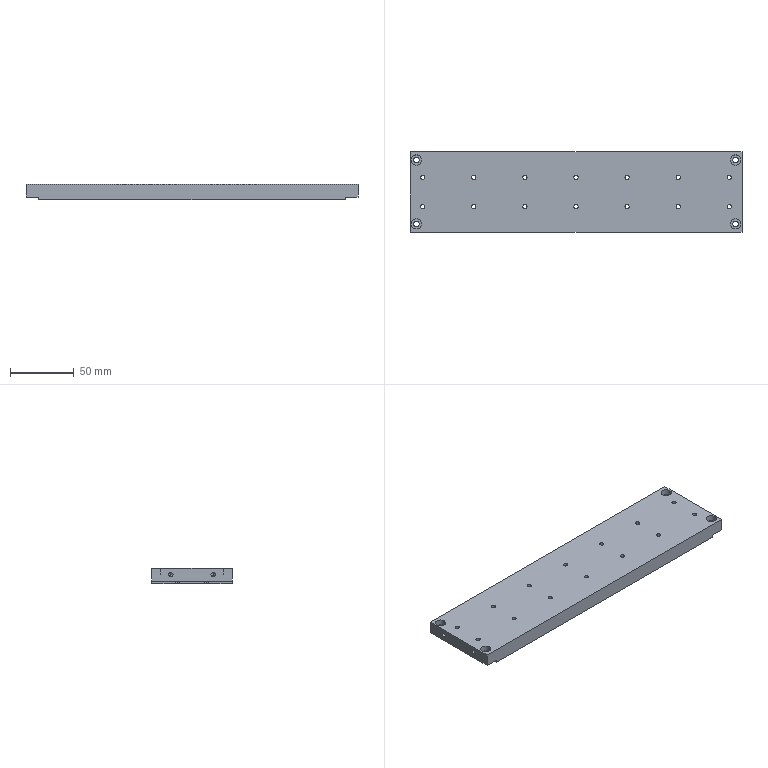Part | STEP file | 2032 Upper mounting plate on base | 1 solid | 78 faces | box 260 x 63 x 12 mm | volume 190964 mm3 | cylinder 52 | plane 18 | cone 8 | commonest cylinder face diameters 3.3 x36 4.5 x8 8 x8